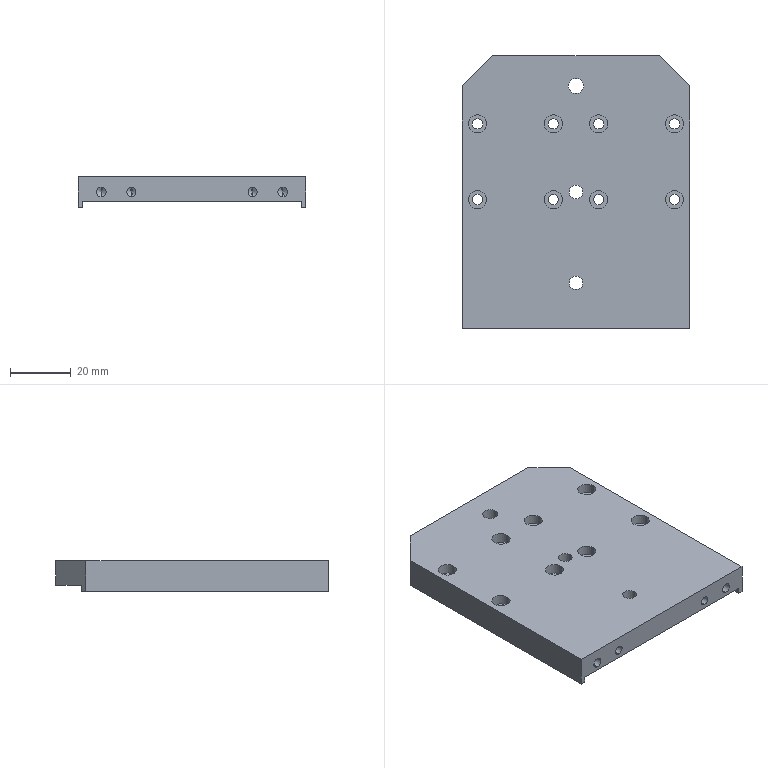Part | STEP file | PN_0044 | 1 solid | 80 faces | box 75 x 90 x 10 mm | volume 51506 mm3 | cylinder 50 | plane 22 | cone 8 | commonest cylinder face diameters 3.4 x16 6 x16 3 x4 3.3 x4 4.5 x4 8 x4